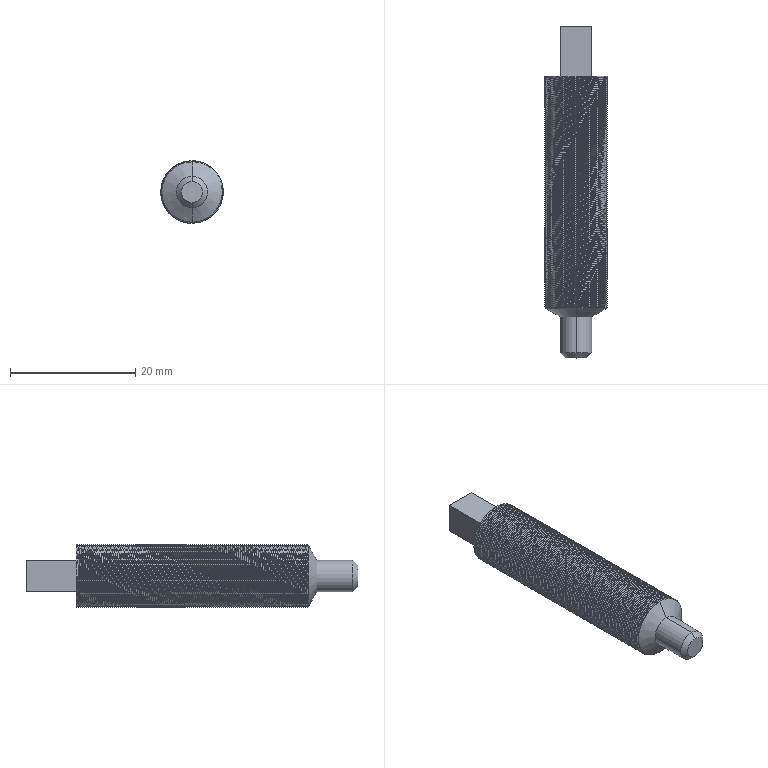Part | SolidWorks | features ICE 1, Revolution 1, SweepThread 1 | 1 solid | 251 faces | box 10 x 53 x 10 mm | volume 3177 mm3 | cylinder 236 | plane 8 | cone 4 | spline 3 | commonest cylinder face diameters 10 x234 5 x2